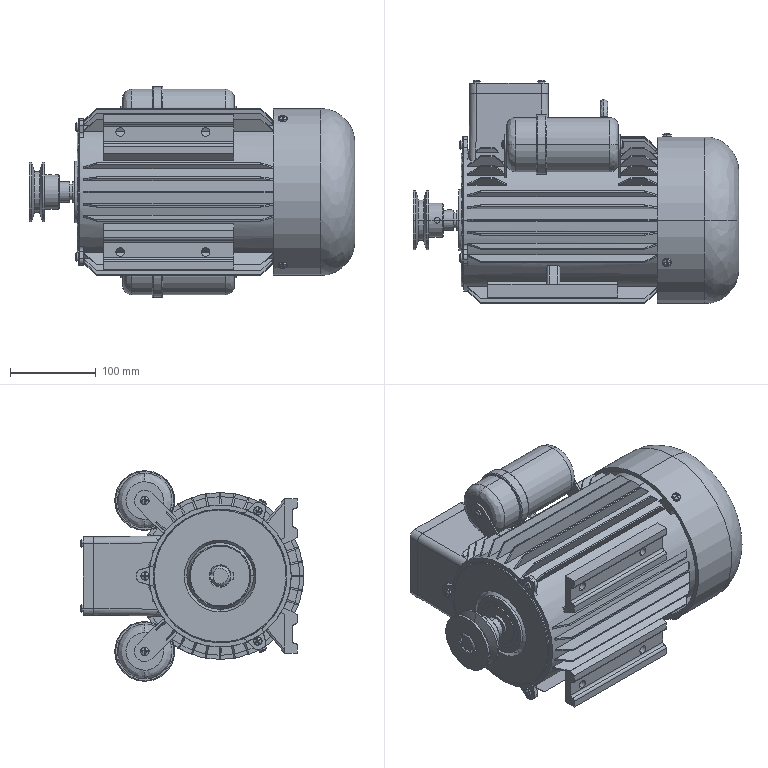Part | SolidWorks | 5 solids | 770 faces | box 380 x 260.832 x 246 mm | volume 9284753 mm3 | plane 391 | cylinder 194 | cone 99 | spline 86 | commonest cylinder face diameters 10 x56 195 x51 24 x13 5.625 x12 8.444 x8 16 x8